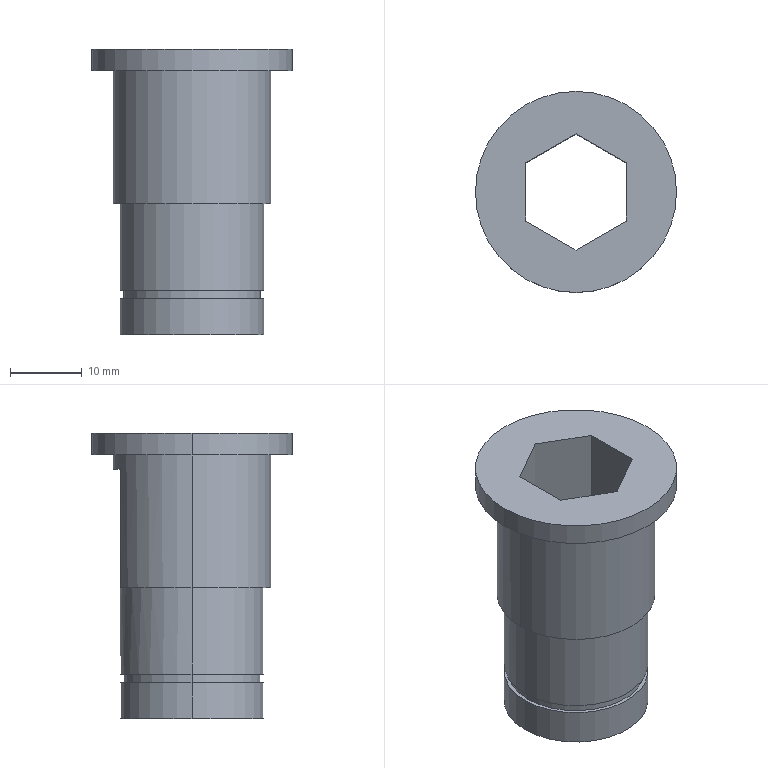Part | SolidWorks | features ICE 5, Extrusion 1, RevCut 1 | 1 solid | 24 faces | box 28 x 28 x 39.7 mm | volume 7720 mm3 | plane 14 | cylinder 10 | commonest cylinder face diameters 20 x4 19 x2 22 x2 28 x2
STEP:
#1=CARTESIAN_POINT('',(-9.5,0.,3.5));
#2=VERTEX_POINT('',#1);
#3=CARTESIAN_POINT('',(9.5,0.,3.5));
#4=VERTEX_POINT('',#3);
#5=CARTESIAN_POINT('',(0.,0.,3.5));
#6=DIRECTION('',(0.,0.,-1.));
#7=DIRECTION('',(-1.,0.,0.));
#8=AXIS2_PLACEMENT_3D('',#5,#6,#7);
#9=CIRCLE('',#8,9.5);
#10=EDGE_CURVE('',#2,#4,#9,.T.);
#11=ORIENTED_EDGE('',*,*,#10,.T.);
#12=CARTESIAN_POINT('',(9.5,0.,2.3));
#13=VERTEX_POINT('',#12);
#14=CARTESIAN_POINT('',(9.5,0.,-1.695));
#15=DIRECTION('',(0.,0.,-1.));
#16=VECTOR('',#15,1000.);
#17=LINE('',#14,#16);
#18=EDGE_CURVE('',#4,#13,#17,.T.);
#19=ORIENTED_EDGE('',*,*,#18,.T.);
#20=CARTESIAN_POINT('',(-9.5,0.,2.3));
#21=VERTEX_POINT('',#20);
#22=CARTESIAN_POINT('',(0.,0.,2.3));
#23=DIRECTION('',(0.,0.,-1.));
#24=DIRECTION('',(-1.,0.,0.));
#25=AXIS2_PLACEMENT_3D('',#22,#23,#24);
#26=CIRCLE('',#25,9.5);
#27=EDGE_CURVE('',#21,#13,#26,.T.);
#28=ORIENTED_EDGE('',*,*,#27,.F.);
#29=CARTESIAN_POINT('',(-9.5,0.,-1.695));
#30=DIRECTION('',(0.,0.,-1.));
#31=VECTOR('',#30,1000.);
#32=LINE('',#29,#31);
#33=EDGE_CURVE('',#2,#21,#32,.T.);
#34=ORIENTED_EDGE('',*,*,#33,.F.);
#35=EDGE_LOOP('',(#11,#19,#28,#34));
#36=FACE_OUTER_BOUND('',#35,.T.);
#37=CARTESIAN_POINT('',(0.,0.,-1.695));
#38=DIRECTION('',(0.,0.,-1.));
#39=DIRECTION('',(-1.,0.,0.));
#40=AXIS2_PLACEMENT_3D('',#37,#38,#39);
#41=CYLINDRICAL_SURFACE('',#40,9.5);
#42=ADVANCED_FACE('',(#36),#41,.T.);
#43=CARTESIAN_POINT('',(14.,0.,37.));
#44=VERTEX_POINT('',#43);
#45=CARTESIAN_POINT('',(-14.,0.,37.));
#46=VERTEX_POINT('',#45);
#47=CARTESIAN_POINT('',(0.,0.,37.));
#48=DIRECTION('',(0.,0.,1.));
#49=DIRECTION('',(1.,0.,0.));
#50=AXIS2_PLACEMENT_3D('',#47,#48,#49);
#51=CIRCLE('',#50,14.);
#52=EDGE_CURVE('',#44,#46,#51,.T.);
#53=ORIENTED_EDGE('',*,*,#52,.F.);
#54=CARTESIAN_POINT('',(14.,0.,34.));
#55=VERTEX_POINT('',#54);
#56=CARTESIAN_POINT('',(14.,0.,37.));
#57=DIRECTION('',(0.,0.,-1.));
#58=VECTOR('',#57,1000.);
#59=LINE('',#56,#58);
#60=EDGE_CURVE('',#44,#55,#59,.T.);
#61=ORIENTED_EDGE('',*,*,#60,.T.);
#62=CARTESIAN_POINT('',(-14.,0.,34.));
#63=VERTEX_POINT('',#62);
#64=CARTESIAN_POINT('',(0.,0.,34.));
#65=DIRECTION('',(0.,0.,1.));
#66=DIRECTION('',(1.,0.,0.));
#67=AXIS2_PLACEMENT_3D('',#64,#65,#66);
#68=CIRCLE('',#67,14.);
#69=EDGE_CURVE('',#55,#63,#68,.T.);
#70=ORIENTED_EDGE('',*,*,#69,.T.);
#71=CARTESIAN_POINT('',(-14.,0.,37.));
#72=DIRECTION('',(0.,0.,-1.));
#73=VECTOR('',#72,1000.);
#74=LINE('',#71,#73);
#75=EDGE_CURVE('',#46,#63,#74,.T.);
#76=ORIENTED_EDGE('',*,*,#75,.F.);
#77=EDGE_LOOP('',(#53,#61,#70,#76));
#78=FACE_OUTER_BOUND('',#77,.T.);
#79=CARTESIAN_POINT('',(0.,0.,37.));
#80=DIRECTION('',(0.,0.,-1.));
#81=DIRECTION('',(-1.,0.,0.));
#82=AXIS2_PLACEMENT_3D('',#79,#80,#81);
#83=CYLINDRICAL_SURFACE('',#82,14.);
#84=ADVANCED_FACE('',(#78),#83,.T.);
#85=CARTESIAN_POINT('',(11.,0.,34.));
#86=VERTEX_POINT('',#85);
#87=CARTESIAN_POINT('',(-11.,0.,34.));
#88=VERTEX_POINT('',#87);
#89=CARTESIAN_POINT('',(0.,0.,34.));
#90=DIRECTION('',(0.,0.,1.));
#91=DIRECTION('',(1.,0.,0.));
#92=AXIS2_PLACEMENT_3D('',#89,#90,#91);
#93=CIRCLE('',#92,11.);
#94=EDGE_CURVE('',#86,#88,#93,.T.);
#95=ORIENTED_EDGE('',*,*,#94,.F.);
#96=CARTESIAN_POINT('',(11.,0.,15.5));
#97=VERTEX_POINT('',#96);
#98=CARTESIAN_POINT('',(11.,0.,34.));
#99=DIRECTION('',(0.,0.,-1.));
#100=VECTOR('',#99,1000.);
#101=LINE('',#98,#100);
#102=EDGE_CURVE('',#86,#97,#101,.T.);
#103=ORIENTED_EDGE('',*,*,#102,.T.);
#104=CARTESIAN_POINT('',(4.583,10.,15.5));
#105=VERTEX_POINT('',#104);
#106=CARTESIAN_POINT('',(0.,0.,15.5));
#107=DIRECTION('',(0.,0.,-1.));
#108=DIRECTION('',(-1.,0.,0.));
#109=AXIS2_PLACEMENT_3D('',#106,#107,#108);
#110=CIRCLE('',#109,11.);
#111=EDGE_CURVE('',#105,#97,#110,.T.);
#112=ORIENTED_EDGE('',*,*,#111,.F.);
#113=CARTESIAN_POINT('',(4.583,10.,32.));
#114=VERTEX_POINT('',#113);
#115=CARTESIAN_POINT('',(4.583,10.,34.));
#116=DIRECTION('',(0.,0.,1.));
#117=VECTOR('',#116,1000.);
#118=LINE('',#115,#117);
#119=EDGE_CURVE('',#105,#114,#118,.T.);
#120=ORIENTED_EDGE('',*,*,#119,.T.);
#121=CARTESIAN_POINT('',(-4.583,10.,32.));
#122=VERTEX_POINT('',#121);
#123=CARTESIAN_POINT('',(0.,0.,32.));
#124=DIRECTION('',(0.,0.,1.));
#125=DIRECTION('',(1.,0.,0.));
#126=AXIS2_PLACEMENT_3D('',#123,#124,#125);
#127=CIRCLE('',#126,11.);
#128=EDGE_CURVE('',#114,#122,#127,.T.);
#129=ORIENTED_EDGE('',*,*,#128,.T.);
#130=CARTESIAN_POINT('',(-4.583,10.,15.5));
#131=VERTEX_POINT('',#130);
#132=CARTESIAN_POINT('',(-4.583,10.,34.));
#133=DIRECTION('',(0.,0.,-1.));
#134=VECTOR('',#133,1000.);
#135=LINE('',#132,#134);
#136=EDGE_CURVE('',#122,#131,#135,.T.);
#137=ORIENTED_EDGE('',*,*,#136,.T.);
#138=CARTESIAN_POINT('',(-11.,0.,15.5));
#139=VERTEX_POINT('',#138);
#140=CARTESIAN_POINT('',(0.,0.,15.5));
#141=DIRECTION('',(0.,0.,-1.));
#142=DIRECTION('',(-1.,0.,0.));
#143=AXIS2_PLACEMENT_3D('',#140,#141,#142);
#144=CIRCLE('',#143,11.);
#145=EDGE_CURVE('',#139,#131,#144,.T.);
#146=ORIENTED_EDGE('',*,*,#145,.F.);
#147=CARTESIAN_POINT('',(-11.,0.,34.));
#148=DIRECTION('',(0.,0.,-1.));
#149=VECTOR('',#148,1000.);
#150=LINE('',#147,#149);
#151=EDGE_CURVE('',#88,#139,#150,.T.);
#152=ORIENTED_EDGE('',*,*,#151,.F.);
#153=EDGE_LOOP('',(#95,#103,#112,#120,#129,#137,#146,#152));
#154=FACE_OUTER_BOUND('',#153,.T.);
#155=CARTESIAN_POINT('',(0.,0.,34.));
#156=DIRECTION('',(0.,0.,-1.));
#157=DIRECTION('',(-1.,0.,0.));
#158=AXIS2_PLACEMENT_3D('',#155,#156,#157);
#159=CYLINDRICAL_SURFACE('',#158,11.);
#160=ADVANCED_FACE('',(#154),#159,.T.);
#161=CARTESIAN_POINT('',(0.,10.,15.5));
#162=VERTEX_POINT('',#161);
#163=CARTESIAN_POINT('',(10.,0.,15.5));
#164=VERTEX_POINT('',#163);
#165=CARTESIAN_POINT('',(0.,0.,15.5));
#166=DIRECTION('',(0.,0.,-1.));
#167=DIRECTION('',(-1.,0.,0.));
#168=AXIS2_PLACEMENT_3D('',#165,#166,#167);
#169=CIRCLE('',#168,10.);
#170=EDGE_CURVE('',#162,#164,#169,.T.);
#171=ORIENTED_EDGE('',*,*,#170,.T.);
#172=CARTESIAN_POINT('',(10.,0.,3.5));
#173=VERTEX_POINT('',#172);
#174=CARTESIAN_POINT('',(10.,0.,15.5));
#175=DIRECTION('',(0.,0.,-1.));
#176=VECTOR('',#175,1000.);
#177=LINE('',#174,#176);
#178=EDGE_CURVE('',#164,#173,#177,.T.);
#179=ORIENTED_EDGE('',*,*,#178,.T.);
#180=CARTESIAN_POINT('',(-10.,0.,3.5));
#181=VERTEX_POINT('',#180);
#182=CARTESIAN_POINT('',(0.,0.,3.5));
#183=DIRECTION('',(0.,0.,1.));
#184=DIRECTION('',(-1.,0.,0.));
#185=AXIS2_PLACEMENT_3D('',#182,#183,#184);
#186=CIRCLE('',#185,10.);
#187=EDGE_CURVE('',#173,#181,#186,.T.);
#188=ORIENTED_EDGE('',*,*,#187,.T.);
#189=CARTESIAN_POINT('',(-10.,0.,15.5));
#190=VERTEX_POINT('',#189);
#191=CARTESIAN_POINT('',(-10.,0.,15.5));
#192=DIRECTION('',(0.,0.,-1.));
#193=VECTOR('',#192,1000.);
#194=LINE('',#191,#193);
#195=EDGE_CURVE('',#190,#181,#194,.T.);
#196=ORIENTED_EDGE('',*,*,#195,.F.);
#197=CARTESIAN_POINT('',(0.,0.,15.5));
#198=DIRECTION('',(0.,0.,-1.));
#199=DIRECTION('',(-1.,0.,0.));
#200=AXIS2_PLACEMENT_3D('',#197,#198,#199);
#201=CIRCLE('',#200,10.);
#202=EDGE_CURVE('',#190,#162,#201,.T.);
#203=ORIENTED_EDGE('',*,*,#202,.T.);
#204=EDGE_LOOP('',(#171,#179,#188,#196,#203));
#205=FACE_OUTER_BOUND('',#204,.T.);
#206=CARTESIAN_POINT('',(0.,0.,15.5));
#207=DIRECTION('',(0.,0.,-1.));
#208=DIRECTION('',(-1.,0.,0.));
#209=AXIS2_PLACEMENT_3D('',#206,#207,#208);
#210=CYLINDRICAL_SURFACE('',#209,10.);
#211=ADVANCED_FACE('',(#205),#210,.T.);
#212=CARTESIAN_POINT('',(-10.,0.,2.3));
#213=VERTEX_POINT('',#212);
#214=CARTESIAN_POINT('',(10.,0.,2.3));
#215=VERTEX_POINT('',#214);
#216=CARTESIAN_POINT('',(0.,0.,2.3));
#217=DIRECTION('',(0.,0.,-1.));
#218=DIRECTION('',(1.,0.,0.));
#219=AXIS2_PLACEMENT_3D('',#216,#217,#218);
#220=CIRCLE('',#219,10.);
#221=EDGE_CURVE('',#213,#215,#220,.T.);
#222=ORIENTED_EDGE('',*,*,#221,.T.);
#223=CARTESIAN_POINT('',(10.,0.,-2.7));
#224=VERTEX_POINT('',#223);
#225=CARTESIAN_POINT('',(10.,0.,15.5));
#226=DIRECTION('',(0.,0.,-1.));
#227=VECTOR('',#226,1000.);
#228=LINE('',#225,#227);
#229=EDGE_CURVE('',#215,#224,#228,.T.);
#230=ORIENTED_EDGE('',*,*,#229,.T.);
#231=CARTESIAN_POINT('',(-10.,0.,-2.7));
#232=VERTEX_POINT('',#231);
#233=CARTESIAN_POINT('',(0.,0.,-2.7));
#234=DIRECTION('',(0.,0.,-1.));
#235=DIRECTION('',(-1.,0.,0.));
#236=AXIS2_PLACEMENT_3D('',#233,#234,#235);
#237=CIRCLE('',#236,10.);
#238=EDGE_CURVE('',#232,#224,#237,.T.);
#239=ORIENTED_EDGE('',*,*,#238,.F.);
#240=CARTESIAN_POINT('',(-10.,0.,15.5));
#241=DIRECTION('',(0.,0.,-1.));
#242=VECTOR('',#241,1000.);
#243=LINE('',#240,#242);
#244=EDGE_CURVE('',#213,#232,#243,.T.);
#245=ORIENTED_EDGE('',*,*,#244,.F.);
#246=EDGE_LOOP('',(#222,#230,#239,#245));
#247=FACE_OUTER_BOUND('',#246,.T.);
#248=CARTESIAN_POINT('',(0.,0.,15.5));
#249=DIRECTION('',(0.,0.,-1.));
#250=DIRECTION('',(-1.,0.,0.));
#251=AXIS2_PLACEMENT_3D('',#248,#249,#250);
#252=CYLINDRICAL_SURFACE('',#251,10.);
#253=ADVANCED_FACE('',(#247),#252,.T.);
#254=ORIENTED_EDGE('',*,*,#229,.F.);
#255=CARTESIAN_POINT('',(0.,0.,2.3));
#256=DIRECTION('',(0.,0.,-1.));
#257=DIRECTION('',(1.,0.,0.));
#258=AXIS2_PLACEMENT_3D('',#255,#256,#257);
#259=CIRCLE('',#258,10.);
#260=EDGE_CURVE('',#215,#213,#259,.T.);
#261=ORIENTED_EDGE('',*,*,#260,.T.);
#262=ORIENTED_EDGE('',*,*,#244,.T.);
#263=CARTESIAN_POINT('',(0.,0.,-2.7));
#264=DIRECTION('',(0.,0.,-1.));
#265=DIRECTION('',(-1.,0.,0.));
#266=AXIS2_PLACEMENT_3D('',#263,#264,#265);
#267=CIRCLE('',#266,10.);
#268=EDGE_CURVE('',#224,#232,#267,.T.);
#269=ORIENTED_EDGE('',*,*,#268,.F.);
#270=EDGE_LOOP('',(#254,#261,#262,#269));
#271=FACE_OUTER_BOUND('',#270,.T.);
#272=CARTESIAN_POINT('',(0.,0.,15.5));
#273=DIRECTION('',(0.,0.,-1.));
#274=DIRECTION('',(-1.,0.,0.));
#275=AXIS2_PLACEMENT_3D('',#272,#273,#274);
#276=CYLINDRICAL_SURFACE('',#275,10.);
#277=ADVANCED_FACE('',(#271),#276,.T.);
#278=ORIENTED_EDGE('',*,*,#178,.F.);
#279=CARTESIAN_POINT('',(0.,0.,15.5));
#280=DIRECTION('',(0.,0.,-1.));
#281=DIRECTION('',(-1.,0.,0.));
#282=AXIS2_PLACEMENT_3D('',#279,#280,#281);
#283=CIRCLE('',#282,10.);
#284=EDGE_CURVE('',#164,#190,#283,.T.);
#285=ORIENTED_EDGE('',*,*,#284,.T.);
#286=ORIENTED_EDGE('',*,*,#195,.T.);
#287=CARTESIAN_POINT('',(0.,0.,3.5));
#288=DIRECTION('',(0.,0.,1.));
#289=DIRECTION('',(-1.,0.,0.));
#290=AXIS2_PLACEMENT_3D('',#287,#288,#289);
#291=CIRCLE('',#290,10.);
#292=EDGE_CURVE('',#181,#173,#291,.T.);
#293=ORIENTED_EDGE('',*,*,#292,.T.);
#294=EDGE_LOOP('',(#278,#285,#286,#293));
#295=FACE_OUTER_BOUND('',#294,.T.);
#296=CARTESIAN_POINT('',(0.,0.,15.5));
#297=DIRECTION('',(0.,0.,-1.));
#298=DIRECTION('',(-1.,0.,0.));
#299=AXIS2_PLACEMENT_3D('',#296,#297,#298);
#300=CYLINDRICAL_SURFACE('',#299,10.);
#301=ADVANCED_FACE('',(#295),#300,.T.);
#302=ORIENTED_EDGE('',*,*,#102,.F.);
#303=CARTESIAN_POINT('',(0.,0.,34.));
#304=DIRECTION('',(0.,0.,1.));
#305=DIRECTION('',(1.,0.,0.));
#306=AXIS2_PLACEMENT_3D('',#303,#304,#305);
#307=CIRCLE('',#306,11.);
#308=EDGE_CURVE('',#88,#86,#307,.T.);
#309=ORIENTED_EDGE('',*,*,#308,.F.);
#310=ORIENTED_EDGE('',*,*,#151,.T.);
#311=CARTESIAN_POINT('',(0.,0.,15.5));
#312=DIRECTION('',(0.,0.,-1.));
#313=DIRECTION('',(-1.,0.,0.));
#314=AXIS2_PLACEMENT_3D('',#311,#312,#313);
#315=CIRCLE('',#314,11.);
#316=EDGE_CURVE('',#97,#139,#315,.T.);
#317=ORIENTED_EDGE('',*,*,#316,.F.);
#318=EDGE_LOOP('',(#302,#309,#310,#317));
#319=FACE_OUTER_BOUND('',#318,.T.);
#320=CARTESIAN_POINT('',(0.,0.,34.));
#321=DIRECTION('',(0.,0.,-1.));
#322=DIRECTION('',(-1.,0.,0.));
#323=AXIS2_PLACEMENT_3D('',#320,#321,#322);
#324=CYLINDRICAL_SURFACE('',#323,11.);
#325=ADVANCED_FACE('',(#319),#324,.T.);
#326=CARTESIAN_POINT('',(0.,0.,34.));
#327=DIRECTION('',(0.,0.,1.));
#328=DIRECTION('',(1.,0.,0.));
#329=AXIS2_PLACEMENT_3D('',#326,#327,#328);
#330=CIRCLE('',#329,14.);
#331=EDGE_CURVE('',#63,#55,#330,.T.);
#332=ORIENTED_EDGE('',*,*,#331,.F.);
#333=ORIENTED_EDGE('',*,*,#69,.F.);
#334=EDGE_LOOP('',(#332,#333));
#335=FACE_OUTER_BOUND('',#334,.T.);
#336=ORIENTED_EDGE('',*,*,#308,.T.);
#337=ORIENTED_EDGE('',*,*,#94,.T.);
#338=EDGE_LOOP('',(#336,#337));
#339=FACE_BOUND('',#338,.T.);
#340=CARTESIAN_POINT('',(0.,0.,34.));
#341=DIRECTION('',(0.,0.,1.));
#342=DIRECTION('',(1.,0.,0.));
#343=AXIS2_PLACEMENT_3D('',#340,#341,#342);
#344=PLANE('',#343);
#345=ADVANCED_FACE('',(#335,#339),#344,.F.);
#346=CARTESIAN_POINT('',(-7.,4.041,37.));
#347=VERTEX_POINT('',#346);
#348=CARTESIAN_POINT('',(-7.,-4.041,37.));
#349=VERTEX_POINT('',#348);
#350=CARTESIAN_POINT('',(-7.,4.041,37.));
#351=DIRECTION('',(0.,-1.,0.));
#352=VECTOR('',#351,1000.);
#353=LINE('',#350,#352);
#354=EDGE_CURVE('',#347,#349,#353,.T.);
#355=ORIENTED_EDGE('',*,*,#354,.F.);
#356=CARTESIAN_POINT('',(0.,8.083,37.));
#357=VERTEX_POINT('',#356);
#358=CARTESIAN_POINT('',(0.,8.083,37.));
#359=DIRECTION('',(-0.866,-0.5,0.));
#360=VECTOR('',#359,1000.);
#361=LINE('',#358,#360);
#362=EDGE_CURVE('',#357,#347,#361,.T.);
#363=ORIENTED_EDGE('',*,*,#362,.F.);
#364=CARTESIAN_POINT('',(7.,4.041,37.));
#365=VERTEX_POINT('',#364);
#366=CARTESIAN_POINT('',(7.,4.041,37.));
#367=DIRECTION('',(-0.866,0.5,0.));
#368=VECTOR('',#367,1000.);
#369=LINE('',#366,#368);
#370=EDGE_CURVE('',#365,#357,#369,.T.);
#371=ORIENTED_EDGE('',*,*,#370,.F.);
#372=CARTESIAN_POINT('',(7.,-4.041,37.));
#373=VERTEX_POINT('',#372);
#374=CARTESIAN_POINT('',(7.,-4.041,37.));
#375=DIRECTION('',(0.,1.,0.));
#376=VECTOR('',#375,1000.);
#377=LINE('',#374,#376);
#378=EDGE_CURVE('',#373,#365,#377,.T.);
#379=ORIENTED_EDGE('',*,*,#378,.F.);
#380=CARTESIAN_POINT('',(0.,-8.083,37.));
#381=VERTEX_POINT('',#380);
#382=CARTESIAN_POINT('',(0.,-8.083,37.));
#383=DIRECTION('',(0.866,0.5,0.));
#384=VECTOR('',#383,1000.);
#385=LINE('',#382,#384);
#386=EDGE_CURVE('',#381,#373,#385,.T.);
#387=ORIENTED_EDGE('',*,*,#386,.F.);
#388=CARTESIAN_POINT('',(-7.,-4.041,37.));
#389=DIRECTION('',(0.866,-0.5,0.));
#390=VECTOR('',#389,1000.);
#391=LINE('',#388,#390);
#392=EDGE_CURVE('',#349,#381,#391,.T.);
#393=ORIENTED_EDGE('',*,*,#392,.F.);
#394=EDGE_LOOP('',(#355,#363,#371,#379,#387,#393));
#395=FACE_BOUND('',#394,.T.);
#396=CARTESIAN_POINT('',(0.,0.,37.));
#397=DIRECTION('',(0.,0.,1.));
#398=DIRECTION('',(1.,0.,0.));
#399=AXIS2_PLACEMENT_3D('',#396,#397,#398);
#400=CIRCLE('',#399,14.);
#401=EDGE_CURVE('',#46,#44,#400,.T.);
#402=ORIENTED_EDGE('',*,*,#401,.T.);
#403=ORIENTED_EDGE('',*,*,#52,.T.);
#404=EDGE_LOOP('',(#402,#403));
#405=FACE_OUTER_BOUND('',#404,.T.);
#406=CARTESIAN_POINT('',(0.,0.,37.));
#407=DIRECTION('',(0.,0.,1.));
#408=DIRECTION('',(1.,0.,0.));
#409=AXIS2_PLACEMENT_3D('',#406,#407,#408);
#410=PLANE('',#409);
#411=ADVANCED_FACE('',(#395,#405),#410,.T.);
#412=ORIENTED_EDGE('',*,*,#60,.F.);
#413=ORIENTED_EDGE('',*,*,#401,.F.);
#414=ORIENTED_EDGE('',*,*,#75,.T.);
#415=ORIENTED_EDGE('',*,*,#331,.T.);
#416=EDGE_LOOP('',(#412,#413,#414,#415));
#417=FACE_OUTER_BOUND('',#416,.T.);
#418=CARTESIAN_POINT('',(0.,0.,37.));
#419=DIRECTION('',(0.,0.,-1.));
#420=DIRECTION('',(-1.,0.,0.));
#421=AXIS2_PLACEMENT_3D('',#418,#419,#420);
#422=CYLINDRICAL_SURFACE('',#421,14.);
#423=ADVANCED_FACE('',(#417),#422,.T.);
#424=CARTESIAN_POINT('',(0.,10.,15.5));
#425=DIRECTION('',(-1.,0.,0.));
#426=VECTOR('',#425,1000.);
#427=LINE('',#424,#426);
#428=EDGE_CURVE('',#105,#162,#427,.T.);
#429=ORIENTED_EDGE('',*,*,#428,.F.);
#430=ORIENTED_EDGE('',*,*,#111,.T.);
#431=ORIENTED_EDGE('',*,*,#316,.T.);
#432=ORIENTED_EDGE('',*,*,#145,.T.);
#433=CARTESIAN_POINT('',(0.,10.,15.5));
#434=DIRECTION('',(-1.,0.,0.));
#435=VECTOR('',#434,1000.);
#436=LINE('',#433,#435);
#437=EDGE_CURVE('',#162,#131,#436,.T.);
#438=ORIENTED_EDGE('',*,*,#437,.F.);
#439=ORIENTED_EDGE('',*,*,#202,.F.);
#440=ORIENTED_EDGE('',*,*,#284,.F.);
#441=ORIENTED_EDGE('',*,*,#170,.F.);
#442=EDGE_LOOP('',(#429,#430,#431,#432,#438,#439,#440,#441));
#443=FACE_OUTER_BOUND('',#442,.T.);
#444=CARTESIAN_POINT('',(0.,0.,15.5));
#445=DIRECTION('',(0.,0.,-1.));
#446=DIRECTION('',(-1.,0.,0.));
#447=AXIS2_PLACEMENT_3D('',#444,#445,#446);
#448=PLANE('',#447);
#449=ADVANCED_FACE('',(#443),#448,.T.);
#450=CARTESIAN_POINT('',(-7.816,10.,32.));
#451=DIRECTION('',(-1.,0.,0.));
#452=VECTOR('',#451,1000.);
#453=LINE('',#450,#452);
#454=EDGE_CURVE('',#114,#122,#453,.T.);
#455=ORIENTED_EDGE('',*,*,#454,.T.);
#456=ORIENTED_EDGE('',*,*,#128,.F.);
#457=EDGE_LOOP('',(#455,#456));
#458=FACE_OUTER_BOUND('',#457,.T.);
#459=CARTESIAN_POINT('',(0.,0.,32.));
#460=DIRECTION('',(0.,0.,1.));
#461=DIRECTION('',(1.,0.,0.));
#462=AXIS2_PLACEMENT_3D('',#459,#460,#461);
#463=PLANE('',#462);
#464=ADVANCED_FACE('',(#458),#463,.F.);
#465=ORIENTED_EDGE('',*,*,#428,.T.);
#466=ORIENTED_EDGE('',*,*,#437,.T.);
#467=ORIENTED_EDGE('',*,*,#136,.F.);
#468=ORIENTED_EDGE('',*,*,#454,.F.);
#469=ORIENTED_EDGE('',*,*,#119,.F.);
#470=EDGE_LOOP('',(#465,#466,#467,#468,#469));
#471=FACE_OUTER_BOUND('',#470,.T.);
#472=CARTESIAN_POINT('',(-7.816,10.,32.));
#473=DIRECTION('',(0.,-1.,0.));
#474=DIRECTION('',(0.,0.,-1.));
#475=AXIS2_PLACEMENT_3D('',#472,#473,#474);
#476=PLANE('',#475);
#477=ADVANCED_FACE('',(#471),#476,.F.);
#478=ORIENTED_EDGE('',*,*,#386,.T.);
#479=CARTESIAN_POINT('',(7.,-4.041,-2.7));
#480=VERTEX_POINT('',#479);
#481=CARTESIAN_POINT('',(7.,-4.041,0.));
#482=DIRECTION('',(0.,0.,1.));
#483=VECTOR('',#482,1000.);
#484=LINE('',#481,#483);
#485=EDGE_CURVE('',#480,#373,#484,.T.);
#486=ORIENTED_EDGE('',*,*,#485,.F.);
#487=CARTESIAN_POINT('',(0.,-8.083,-2.7));
#488=VERTEX_POINT('',#487);
#489=CARTESIAN_POINT('',(7.,-4.041,-2.7));
#490=DIRECTION('',(-0.866,-0.5,0.));
#491=VECTOR('',#490,1000.);
#492=LINE('',#489,#491);
#493=EDGE_CURVE('',#480,#488,#492,.T.);
#494=ORIENTED_EDGE('',*,*,#493,.T.);
#495=CARTESIAN_POINT('',(0.,-8.083,0.));
#496=DIRECTION('',(0.,0.,1.));
#497=VECTOR('',#496,1000.);
#498=LINE('',#495,#497);
#499=EDGE_CURVE('',#488,#381,#498,.T.);
#500=ORIENTED_EDGE('',*,*,#499,.T.);
#501=EDGE_LOOP('',(#478,#486,#494,#500));
#502=FACE_OUTER_BOUND('',#501,.T.);
#503=CARTESIAN_POINT('',(0.,-8.083,0.));
#504=DIRECTION('',(0.5,-0.866,0.));
#505=DIRECTION('',(0.866,0.5,0.));
#506=AXIS2_PLACEMENT_3D('',#503,#504,#505);
#507=PLANE('',#506);
#508=ADVANCED_FACE('',(#502),#507,.F.);
#509=ORIENTED_EDGE('',*,*,#392,.T.);
#510=ORIENTED_EDGE('',*,*,#499,.F.);
#511=CARTESIAN_POINT('',(-7.,-4.041,-2.7));
#512=VERTEX_POINT('',#511);
#513=CARTESIAN_POINT('',(0.,-8.083,-2.7));
#514=DIRECTION('',(-0.866,0.5,0.));
#515=VECTOR('',#514,1000.);
#516=LINE('',#513,#515);
#517=EDGE_CURVE('',#488,#512,#516,.T.);
#518=ORIENTED_EDGE('',*,*,#517,.T.);
#519=CARTESIAN_POINT('',(-7.,-4.041,0.));
#520=DIRECTION('',(0.,0.,1.));
#521=VECTOR('',#520,1000.);
#522=LINE('',#519,#521);
#523=EDGE_CURVE('',#512,#349,#522,.T.);
#524=ORIENTED_EDGE('',*,*,#523,.T.);
#525=EDGE_LOOP('',(#509,#510,#518,#524));
#526=FACE_OUTER_BOUND('',#525,.T.);
#527=CARTESIAN_POINT('',(-7.,-4.041,0.));
#528=DIRECTION('',(-0.5,-0.866,0.));
#529=DIRECTION('',(0.866,-0.5,0.));
#530=AXIS2_PLACEMENT_3D('',#527,#528,#529);
#531=PLANE('',#530);
#532=ADVANCED_FACE('',(#526),#531,.F.);
#533=ORIENTED_EDGE('',*,*,#354,.T.);
#534=ORIENTED_EDGE('',*,*,#523,.F.);
#535=CARTESIAN_POINT('',(-7.,4.041,-2.7));
#536=VERTEX_POINT('',#535);
#537=CARTESIAN_POINT('',(-7.,-4.041,-2.7));
#538=DIRECTION('',(0.,1.,0.));
#539=VECTOR('',#538,1000.);
#540=LINE('',#537,#539);
#541=EDGE_CURVE('',#512,#536,#540,.T.);
#542=ORIENTED_EDGE('',*,*,#541,.T.);
#543=CARTESIAN_POINT('',(-7.,4.041,0.));
#544=DIRECTION('',(0.,0.,1.));
#545=VECTOR('',#544,1000.);
#546=LINE('',#543,#545);
#547=EDGE_CURVE('',#536,#347,#546,.T.);
#548=ORIENTED_EDGE('',*,*,#547,.T.);
#549=EDGE_LOOP('',(#533,#534,#542,#548));
#550=FACE_OUTER_BOUND('',#549,.T.);
#551=CARTESIAN_POINT('',(-7.,4.041,0.));
#552=DIRECTION('',(-1.,0.,0.));
#553=DIRECTION('',(0.,-1.,0.));
#554=AXIS2_PLACEMENT_3D('',#551,#552,#553);
#555=PLANE('',#554);
#556=ADVANCED_FACE('',(#550),#555,.F.);
#557=ORIENTED_EDGE('',*,*,#362,.T.);
#558=ORIENTED_EDGE('',*,*,#547,.F.);
#559=CARTESIAN_POINT('',(0.,8.083,-2.7));
#560=VERTEX_POINT('',#559);
#561=CARTESIAN_POINT('',(-7.,4.041,-2.7));
#562=DIRECTION('',(0.866,0.5,0.));
#563=VECTOR('',#562,1000.);
#564=LINE('',#561,#563);
#565=EDGE_CURVE('',#536,#560,#564,.T.);
#566=ORIENTED_EDGE('',*,*,#565,.T.);
#567=CARTESIAN_POINT('',(0.,8.083,0.));
#568=DIRECTION('',(0.,0.,1.));
#569=VECTOR('',#568,1000.);
#570=LINE('',#567,#569);
#571=EDGE_CURVE('',#560,#357,#570,.T.);
#572=ORIENTED_EDGE('',*,*,#571,.T.);
#573=EDGE_LOOP('',(#557,#558,#566,#572));
#574=FACE_OUTER_BOUND('',#573,.T.);
#575=CARTESIAN_POINT('',(0.,8.083,0.));
#576=DIRECTION('',(-0.5,0.866,0.));
#577=DIRECTION('',(-0.866,-0.5,0.));
#578=AXIS2_PLACEMENT_3D('',#575,#576,#577);
#579=PLANE('',#578);
#580=ADVANCED_FACE('',(#574),#579,.F.);
#581=ORIENTED_EDGE('',*,*,#370,.T.);
#582=ORIENTED_EDGE('',*,*,#571,.F.);
#583=CARTESIAN_POINT('',(7.,4.041,-2.7));
#584=VERTEX_POINT('',#583);
#585=CARTESIAN_POINT('',(0.,8.083,-2.7));
#586=DIRECTION('',(0.866,-0.5,0.));
#587=VECTOR('',#586,1000.);
#588=LINE('',#585,#587);
#589=EDGE_CURVE('',#560,#584,#588,.T.);
#590=ORIENTED_EDGE('',*,*,#589,.T.);
#591=CARTESIAN_POINT('',(7.,4.041,0.));
#592=DIRECTION('',(0.,0.,1.));
#593=VECTOR('',#592,1000.);
#594=LINE('',#591,#593);
#595=EDGE_CURVE('',#584,#365,#594,.T.);
#596=ORIENTED_EDGE('',*,*,#595,.T.);
#597=EDGE_LOOP('',(#581,#582,#590,#596));
#598=FACE_OUTER_BOUND('',#597,.T.);
#599=CARTESIAN_POINT('',(7.,4.041,0.));
#600=DIRECTION('',(0.5,0.866,0.));
#601=DIRECTION('',(-0.866,0.5,0.));
#602=AXIS2_PLACEMENT_3D('',#599,#600,#601);
#603=PLANE('',#602);
#604=ADVANCED_FACE('',(#598),#603,.F.);
#605=ORIENTED_EDGE('',*,*,#485,.T.);
#606=ORIENTED_EDGE('',*,*,#378,.T.);
#607=ORIENTED_EDGE('',*,*,#595,.F.);
#608=CARTESIAN_POINT('',(7.,4.041,-2.7));
#609=DIRECTION('',(0.,-1.,0.));
#610=VECTOR('',#609,1000.);
#611=LINE('',#608,#610);
#612=EDGE_CURVE('',#584,#480,#611,.T.);
#613=ORIENTED_EDGE('',*,*,#612,.T.);
#614=EDGE_LOOP('',(#605,#606,#607,#613));
#615=FACE_OUTER_BOUND('',#614,.T.);
#616=CARTESIAN_POINT('',(7.,-4.041,0.));
#617=DIRECTION('',(1.,0.,0.));
#618=DIRECTION('',(0.,1.,0.));
#619=AXIS2_PLACEMENT_3D('',#616,#617,#618);
#620=PLANE('',#619);
#621=ADVANCED_FACE('',(#615),#620,.F.);
#622=ORIENTED_EDGE('',*,*,#221,.F.);
#623=ORIENTED_EDGE('',*,*,#260,.F.);
#624=EDGE_LOOP('',(#622,#623));
#625=FACE_OUTER_BOUND('',#624,.T.);
#626=ORIENTED_EDGE('',*,*,#27,.T.);
#627=CARTESIAN_POINT('',(0.,0.,2.3));
#628=DIRECTION('',(0.,0.,-1.));
#629=DIRECTION('',(-1.,0.,0.));
#630=AXIS2_PLACEMENT_3D('',#627,#628,#629);
#631=CIRCLE('',#630,9.5);
#632=EDGE_CURVE('',#13,#21,#631,.T.);
#633=ORIENTED_EDGE('',*,*,#632,.T.);
#634=EDGE_LOOP('',(#626,#633));
#635=FACE_BOUND('',#634,.T.);
#636=CARTESIAN_POINT('',(9.5,0.,2.3));
#637=DIRECTION('',(0.,0.,1.));
#638=DIRECTION('',(1.,0.,0.));
#639=AXIS2_PLACEMENT_3D('',#636,#637,#638);
#640=PLANE('',#639);
#641=ADVANCED_FACE('',(#625,#635),#640,.T.);
#642=ORIENTED_EDGE('',*,*,#18,.F.);
#643=CARTESIAN_POINT('',(0.,0.,3.5));
#644=DIRECTION('',(0.,0.,-1.));
#645=DIRECTION('',(-1.,0.,0.));
#646=AXIS2_PLACEMENT_3D('',#643,#644,#645);
#647=CIRCLE('',#646,9.5);
#648=EDGE_CURVE('',#4,#2,#647,.T.);
#649=ORIENTED_EDGE('',*,*,#648,.T.);
#650=ORIENTED_EDGE('',*,*,#33,.T.);
#651=ORIENTED_EDGE('',*,*,#632,.F.);
#652=EDGE_LOOP('',(#642,#649,#650,#651));
#653=FACE_OUTER_BOUND('',#652,.T.);
#654=CARTESIAN_POINT('',(0.,0.,-1.695));
#655=DIRECTION('',(0.,0.,-1.));
#656=DIRECTION('',(-1.,0.,0.));
#657=AXIS2_PLACEMENT_3D('',#654,#655,#656);
#658=CYLINDRICAL_SURFACE('',#657,9.5);
#659=ADVANCED_FACE('',(#653),#658,.T.);
#660=ORIENTED_EDGE('',*,*,#292,.F.);
#661=ORIENTED_EDGE('',*,*,#187,.F.);
#662=EDGE_LOOP('',(#660,#661));
#663=FACE_OUTER_BOUND('',#662,.T.);
#664=ORIENTED_EDGE('',*,*,#10,.F.);
#665=ORIENTED_EDGE('',*,*,#648,.F.);
#666=EDGE_LOOP('',(#664,#665));
#667=FACE_BOUND('',#666,.T.);
#668=CARTESIAN_POINT('',(9.5,0.,3.5));
#669=DIRECTION('',(0.,0.,-1.));
#670=DIRECTION('',(-1.,0.,0.));
#671=AXIS2_PLACEMENT_3D('',#668,#669,#670);
#672=PLANE('',#671);
#673=ADVANCED_FACE('',(#663,#667),#672,.T.);
#674=ORIENTED_EDGE('',*,*,#238,.T.);
#675=ORIENTED_EDGE('',*,*,#268,.T.);
#676=EDGE_LOOP('',(#674,#675));
#677=FACE_OUTER_BOUND('',#676,.T.);
#678=ORIENTED_EDGE('',*,*,#541,.F.);
#679=ORIENTED_EDGE('',*,*,#517,.F.);
#680=ORIENTED_EDGE('',*,*,#493,.F.);
#681=ORIENTED_EDGE('',*,*,#612,.F.);
#682=ORIENTED_EDGE('',*,*,#589,.F.);
#683=ORIENTED_EDGE('',*,*,#565,.F.);
#684=EDGE_LOOP('',(#678,#679,#680,#681,#682,#683));
#685=FACE_BOUND('',#684,.T.);
#686=CARTESIAN_POINT('',(0.,0.,-2.7));
#687=DIRECTION('',(0.,0.,-1.));
#688=DIRECTION('',(-1.,0.,0.));
#689=AXIS2_PLACEMENT_3D('',#686,#687,#688);
#690=PLANE('',#689);
#691=ADVANCED_FACE('',(#677,#685),#690,.T.);
#692=CLOSED_SHELL('',(#42,#84,#160,#211,#253,#277,#301,#325,#345,#411,#423,#449,#464,#477,#508,#532,#556,#580,#604,#621,#641,#659,#673,#691));
#693=MANIFOLD_SOLID_BREP('',#692);
#694=CARTESIAN_POINT('',(0.,0.,0.));
#695=DIRECTION('',(0.,0.,1.));
#696=DIRECTION('',(1.,0.,0.));
#697=AXIS2_PLACEMENT_3D('',#694,#695,#696);
#698=(LENGTH_UNIT()NAMED_UNIT(*)SI_UNIT(.MILLI.,.METRE.));
#699=UNCERTAINTY_MEASURE_WITH_UNIT(LENGTH_MEASURE(0.00001),#698,'','');
#700=(NAMED_UNIT(*)PLANE_ANGLE_UNIT()SI_UNIT($,.RADIAN.));
#701=(NAMED_UNIT(*)SI_UNIT($,.STERADIAN.)SOLID_ANGLE_UNIT());
#702=(GEOMETRIC_REPRESENTATION_CONTEXT(3)GLOBAL_UNCERTAINTY_ASSIGNED_CONTEXT((#699))GLOBAL_UNIT_ASSIGNED_CONTEXT((#698,#700,#701))REPRESENTATION_CONTEXT('',''));
#703=ADVANCED_BREP_SHAPE_REPRESENTATION('',(#693,#697),#702);